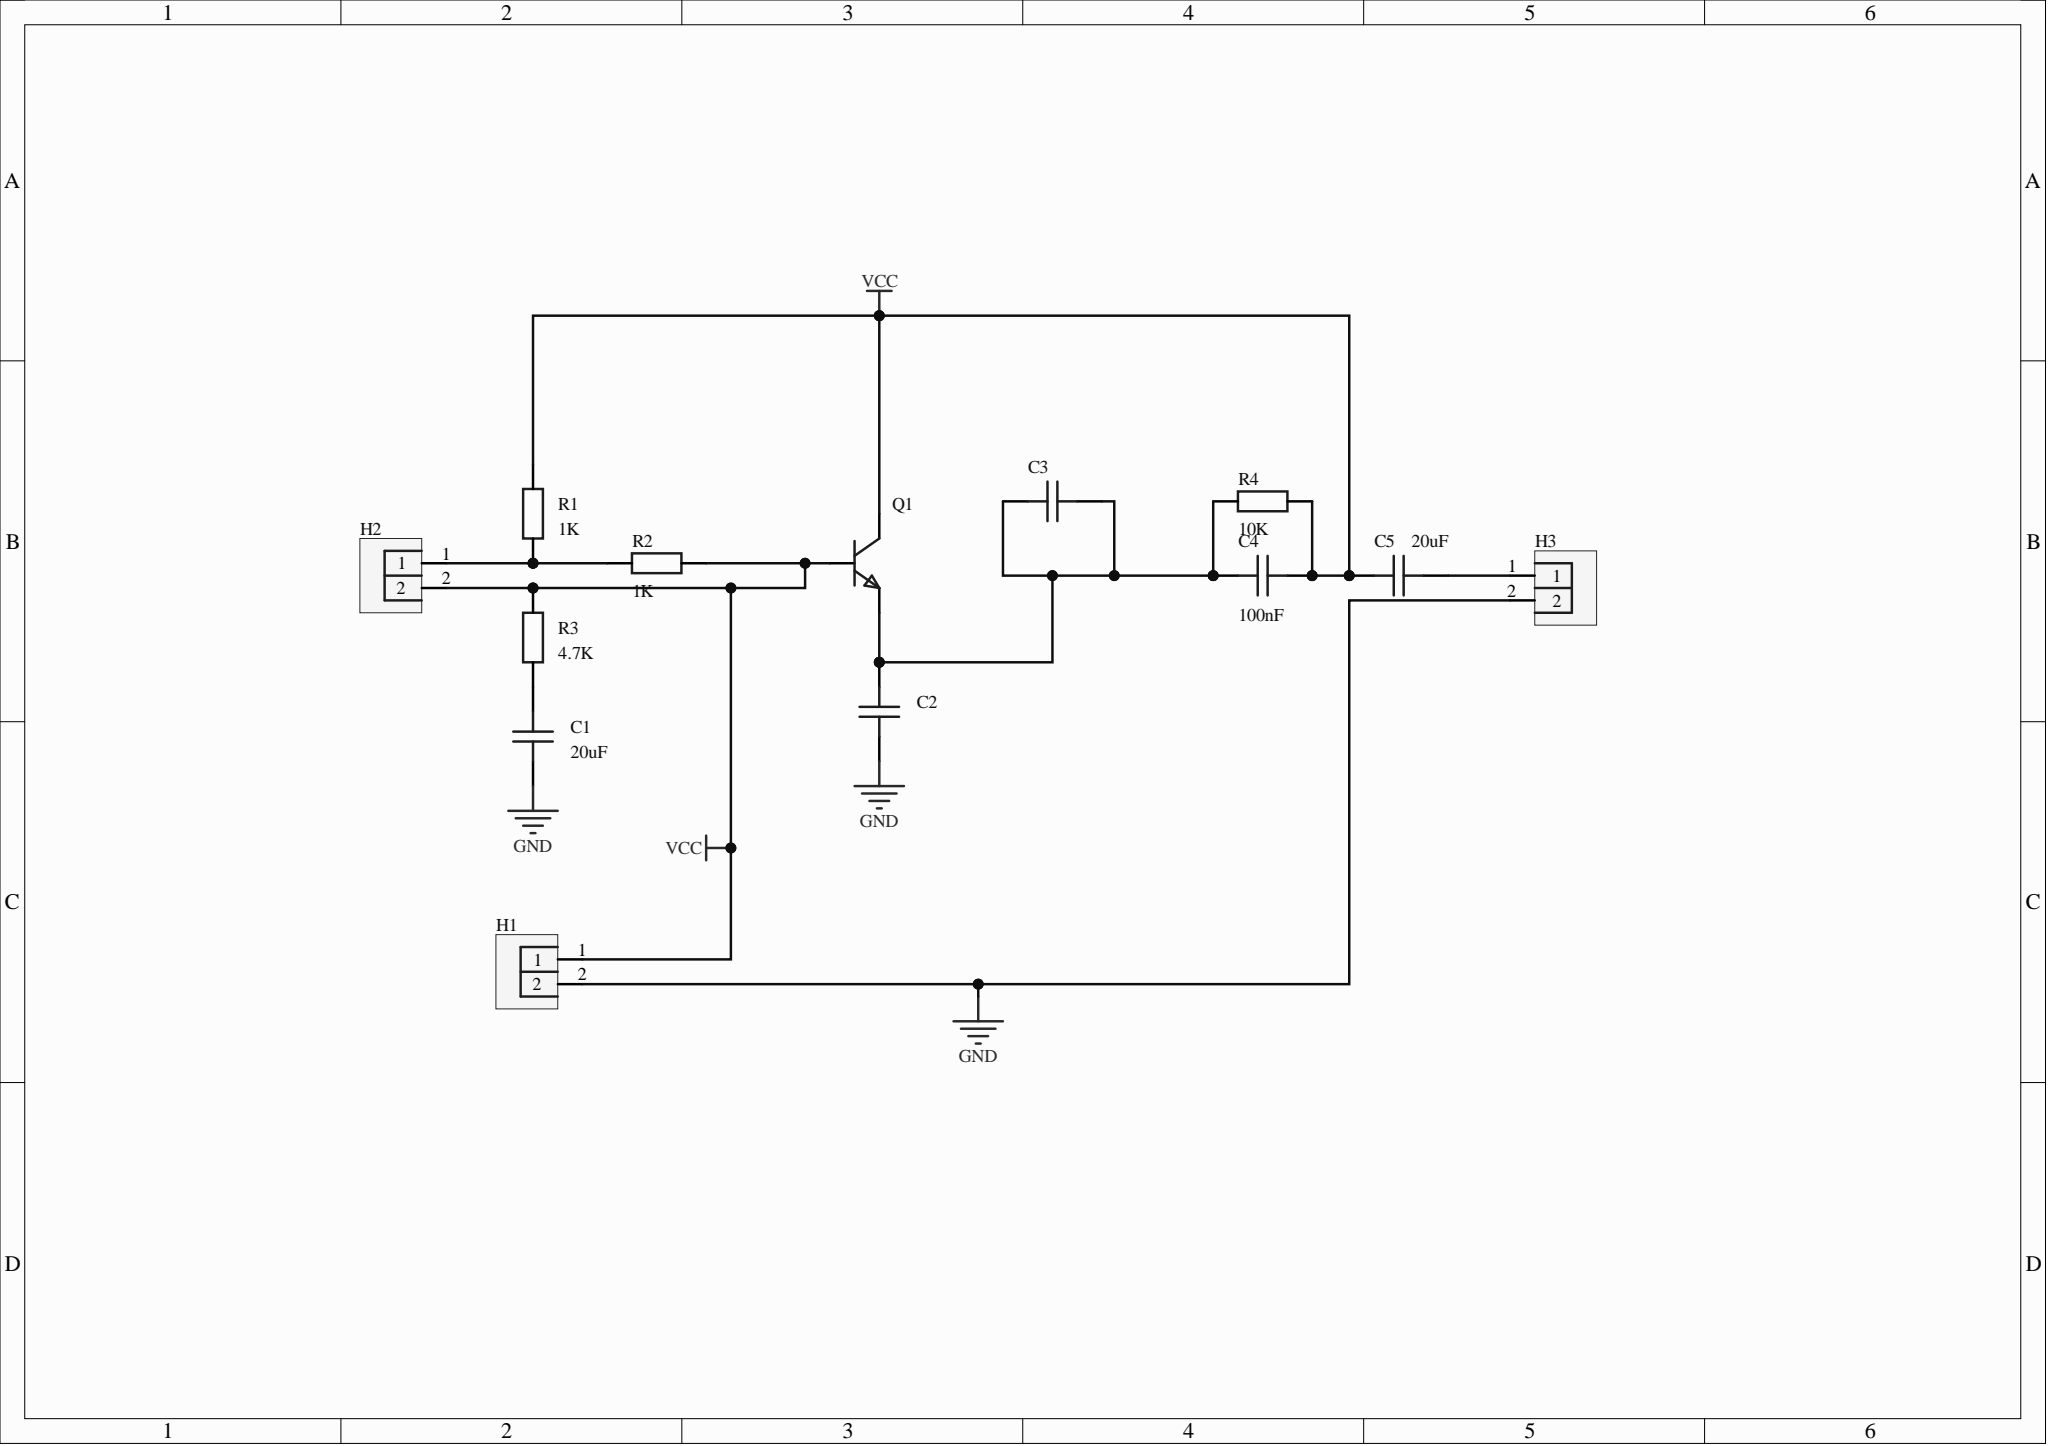Circuit board | Altium Designer | 13 parts | 6 nets
Bill of materials:
Comment,Description,Designator,Footprint,LibRef,Quantity
"20uF","","C1, C5","C0603","CAP_0603","2"
"100nF","","C2, C3, C4","C0603","CAP_0603","3"
"","","H1, H2, H3","HDR-TH_2P-P2.54-V-M-1","HDR-M_2.54_1x2P","3"
"","","Q1","S8050_SOT-23","S8050_SOT_NPN","1"
"1K","","R1, R2","R0603","Res_0603","2"
"4.7K","","R3","R0603","Res_0603","1"
"10K","","R4","R0603","Res_0603","1"
Netlist (Protel format):
[
C1
C0603
20uF



]
[
C2
C0603
100nF



]
[
C3
C0603
100nF



]
[
C4
C0603
100nF



]
[
C5
C0603
20uF



]
[
H1
HDR-TH_2P-P2.54-V-M-1




]
[
H2
HDR-TH_2P-P2.54-V-M-1




]
[
H3
HDR-TH_2P-P2.54-V-M-1




]
[
Q1
S8050_SOT-23




]
[
R1
R0603
1K



]
[
R2
R0603
1K



]
[
R3
R0603
4.7K



]
[
R4
R0603
10K



]
(
VCC
C4-2
C5-1
H1-1
H2-2
Q1-1
Q1-3
R1-2
R2-1
R3-2
R4-2
)
(
NetH2_1
H2-1
R1-1
R2-2
)
(
NetC5_2
C5-2
H3-1
)
(
NetC2_2
C2-2
C3-1
C3-2
C4-1
Q1-2
R4-1
)
(
NetC1_2
C1-2
R3-1
)
(
GND
C1-1
C2-1
H1-2
H3-2
)